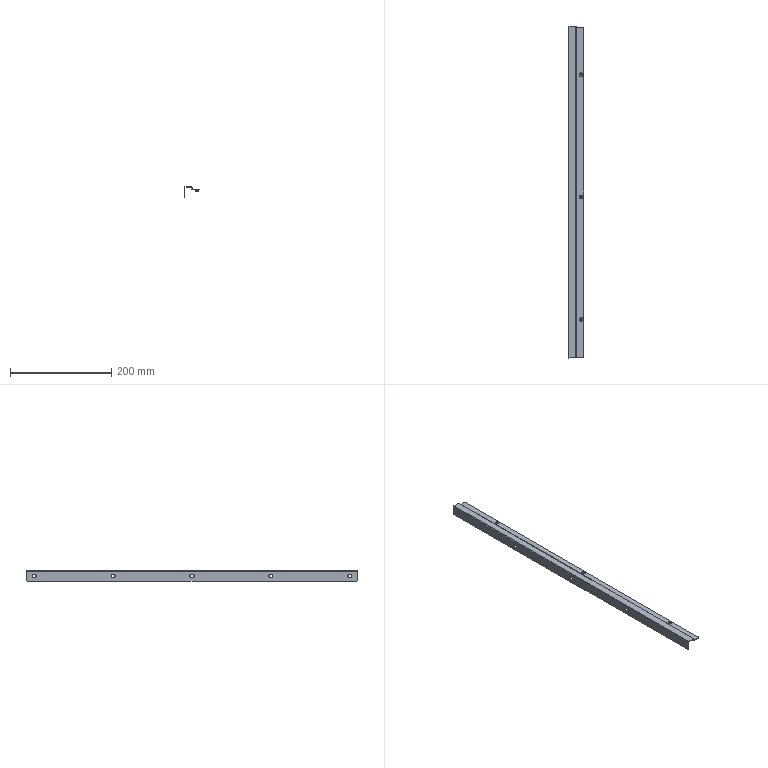Part | STEP file | HESS-408-70-15W-N-12-inner liner closing plate bracket Z | 1 solid | 72 faces | box 30 x 657 x 20 mm | volume 34871 mm3 | cylinder 33 | plane 27 | spline 12 | commonest cylinder face diameters 5 x10 3.2 x6 5.2 x6 6 x4 0.1 x3 2.1 x3